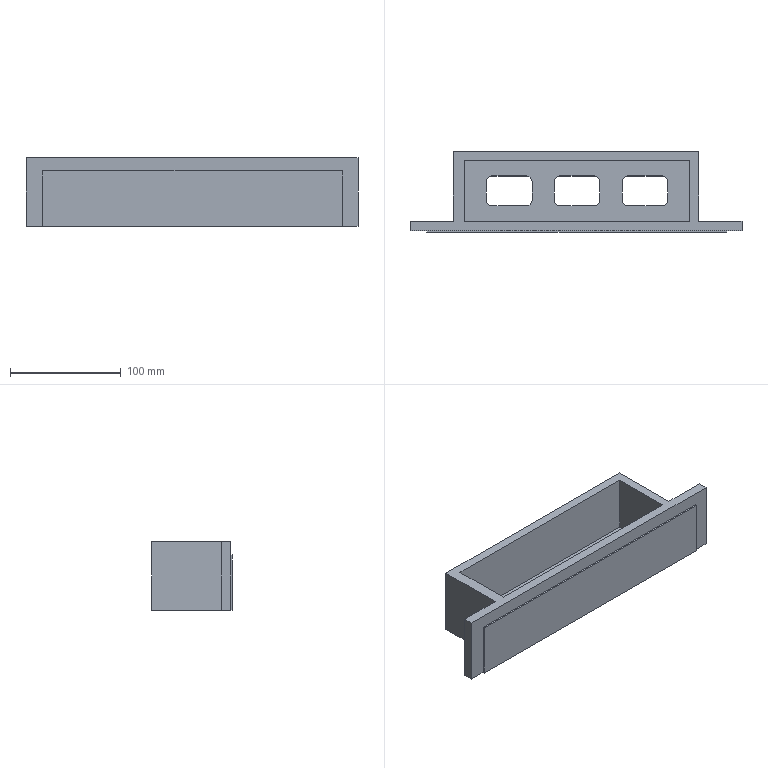Part | SolidWorks | features ICE 6, Extrusion 1, Fillet 1 | 1 solid | 43 faces | box 300 x 73 x 62 mm | volume 429281 mm3 | plane 31 | cylinder 12 | commonest cylinder face diameters 10 x12
STEP:
#1=CARTESIAN_POINT('',(-101.,5.,-21.));
#2=VERTEX_POINT('',#1);
#3=CARTESIAN_POINT('',(103.,5.,-21.));
#4=VERTEX_POINT('',#3);
#5=CARTESIAN_POINT('',(103.,5.,-21.));
#6=DIRECTION('',(1.,0.,0.));
#7=VECTOR('',#6,1000.);
#8=LINE('',#5,#7);
#9=EDGE_CURVE('',#2,#4,#8,.T.);
#10=ORIENTED_EDGE('',*,*,#9,.T.);
#11=CARTESIAN_POINT('',(103.,60.,-21.));
#12=VERTEX_POINT('',#11);
#13=CARTESIAN_POINT('',(103.,60.,-21.));
#14=DIRECTION('',(0.,-1.,0.));
#15=VECTOR('',#14,1000.);
#16=LINE('',#13,#15);
#17=EDGE_CURVE('',#12,#4,#16,.T.);
#18=ORIENTED_EDGE('',*,*,#17,.F.);
#19=CARTESIAN_POINT('',(-101.,60.,-21.));
#20=VERTEX_POINT('',#19);
#21=CARTESIAN_POINT('',(103.,60.,-21.));
#22=DIRECTION('',(1.,0.,0.));
#23=VECTOR('',#22,1000.);
#24=LINE('',#21,#23);
#25=EDGE_CURVE('',#20,#12,#24,.T.);
#26=ORIENTED_EDGE('',*,*,#25,.F.);
#27=CARTESIAN_POINT('',(-101.,60.,-21.));
#28=DIRECTION('',(0.,-1.,0.));
#29=VECTOR('',#28,1000.);
#30=LINE('',#27,#29);
#31=EDGE_CURVE('',#20,#2,#30,.T.);
#32=ORIENTED_EDGE('',*,*,#31,.T.);
#33=EDGE_LOOP('',(#10,#18,#26,#32));
#34=FACE_OUTER_BOUND('',#33,.T.);
#35=CARTESIAN_POINT('',(78.,46.,-21.));
#36=VERTEX_POINT('',#35);
#37=CARTESIAN_POINT('',(46.667,46.,-21.));
#38=VERTEX_POINT('',#37);
#39=CARTESIAN_POINT('',(41.667,46.,-21.));
#40=DIRECTION('',(-1.,0.,0.));
#41=VECTOR('',#40,1000.);
#42=LINE('',#39,#41);
#43=EDGE_CURVE('',#36,#38,#42,.T.);
#44=ORIENTED_EDGE('',*,*,#43,.F.);
#45=CARTESIAN_POINT('',(83.,41.,-21.));
#46=VERTEX_POINT('',#45);
#47=CARTESIAN_POINT('',(78.,41.,-21.));
#48=DIRECTION('',(0.,0.,-1.));
#49=DIRECTION('',(-1.,0.,0.));
#50=AXIS2_PLACEMENT_3D('',#47,#48,#49);
#51=CIRCLE('',#50,5.);
#52=EDGE_CURVE('',#36,#46,#51,.T.);
#53=ORIENTED_EDGE('',*,*,#52,.T.);
#54=CARTESIAN_POINT('',(83.,24.,-21.));
#55=VERTEX_POINT('',#54);
#56=CARTESIAN_POINT('',(83.,19.,-21.));
#57=DIRECTION('',(0.,1.,0.));
#58=VECTOR('',#57,1000.);
#59=LINE('',#56,#58);
#60=EDGE_CURVE('',#55,#46,#59,.T.);
#61=ORIENTED_EDGE('',*,*,#60,.F.);
#62=CARTESIAN_POINT('',(78.,19.,-21.));
#63=VERTEX_POINT('',#62);
#64=CARTESIAN_POINT('',(78.,24.,-21.));
#65=DIRECTION('',(0.,0.,-1.));
#66=DIRECTION('',(-1.,0.,0.));
#67=AXIS2_PLACEMENT_3D('',#64,#65,#66);
#68=CIRCLE('',#67,5.);
#69=EDGE_CURVE('',#55,#63,#68,.T.);
#70=ORIENTED_EDGE('',*,*,#69,.T.);
#71=CARTESIAN_POINT('',(46.667,19.,-21.));
#72=VERTEX_POINT('',#71);
#73=CARTESIAN_POINT('',(41.667,19.,-21.));
#74=DIRECTION('',(1.,0.,0.));
#75=VECTOR('',#74,1000.);
#76=LINE('',#73,#75);
#77=EDGE_CURVE('',#72,#63,#76,.T.);
#78=ORIENTED_EDGE('',*,*,#77,.F.);
#79=CARTESIAN_POINT('',(41.667,24.,-21.));
#80=VERTEX_POINT('',#79);
#81=CARTESIAN_POINT('',(46.667,24.,-21.));
#82=DIRECTION('',(0.,0.,-1.));
#83=DIRECTION('',(-1.,0.,0.));
#84=AXIS2_PLACEMENT_3D('',#81,#82,#83);
#85=CIRCLE('',#84,5.);
#86=EDGE_CURVE('',#72,#80,#85,.T.);
#87=ORIENTED_EDGE('',*,*,#86,.T.);
#88=CARTESIAN_POINT('',(41.667,41.,-21.));
#89=VERTEX_POINT('',#88);
#90=CARTESIAN_POINT('',(41.667,19.,-21.));
#91=DIRECTION('',(0.,-1.,0.));
#92=VECTOR('',#91,1000.);
#93=LINE('',#90,#92);
#94=EDGE_CURVE('',#89,#80,#93,.T.);
#95=ORIENTED_EDGE('',*,*,#94,.F.);
#96=CARTESIAN_POINT('',(46.667,41.,-21.));
#97=DIRECTION('',(0.,0.,-1.));
#98=DIRECTION('',(-1.,0.,0.));
#99=AXIS2_PLACEMENT_3D('',#96,#97,#98);
#100=CIRCLE('',#99,5.);
#101=EDGE_CURVE('',#89,#38,#100,.T.);
#102=ORIENTED_EDGE('',*,*,#101,.T.);
#103=EDGE_LOOP('',(#44,#53,#61,#70,#78,#87,#95,#102));
#104=FACE_BOUND('',#103,.T.);
#105=CARTESIAN_POINT('',(-44.667,46.,-21.));
#106=VERTEX_POINT('',#105);
#107=CARTESIAN_POINT('',(-76.,46.,-21.));
#108=VERTEX_POINT('',#107);
#109=CARTESIAN_POINT('',(-81.,46.,-21.));
#110=DIRECTION('',(-1.,0.,0.));
#111=VECTOR('',#110,1000.);
#112=LINE('',#109,#111);
#113=EDGE_CURVE('',#106,#108,#112,.T.);
#114=ORIENTED_EDGE('',*,*,#113,.F.);
#115=CARTESIAN_POINT('',(-39.667,41.,-21.));
#116=VERTEX_POINT('',#115);
#117=CARTESIAN_POINT('',(-44.667,41.,-21.));
#118=DIRECTION('',(0.,0.,-1.));
#119=DIRECTION('',(-1.,0.,0.));
#120=AXIS2_PLACEMENT_3D('',#117,#118,#119);
#121=CIRCLE('',#120,5.);
#122=EDGE_CURVE('',#106,#116,#121,.T.);
#123=ORIENTED_EDGE('',*,*,#122,.T.);
#124=CARTESIAN_POINT('',(-39.667,24.,-21.));
#125=VERTEX_POINT('',#124);
#126=CARTESIAN_POINT('',(-39.667,19.,-21.));
#127=DIRECTION('',(0.,1.,0.));
#128=VECTOR('',#127,1000.);
#129=LINE('',#126,#128);
#130=EDGE_CURVE('',#125,#116,#129,.T.);
#131=ORIENTED_EDGE('',*,*,#130,.F.);
#132=CARTESIAN_POINT('',(-44.667,19.,-21.));
#133=VERTEX_POINT('',#132);
#134=CARTESIAN_POINT('',(-44.667,24.,-21.));
#135=DIRECTION('',(0.,0.,-1.));
#136=DIRECTION('',(-1.,0.,0.));
#137=AXIS2_PLACEMENT_3D('',#134,#135,#136);
#138=CIRCLE('',#137,5.);
#139=EDGE_CURVE('',#125,#133,#138,.T.);
#140=ORIENTED_EDGE('',*,*,#139,.T.);
#141=CARTESIAN_POINT('',(-76.,19.,-21.));
#142=VERTEX_POINT('',#141);
#143=CARTESIAN_POINT('',(-81.,19.,-21.));
#144=DIRECTION('',(1.,0.,0.));
#145=VECTOR('',#144,1000.);
#146=LINE('',#143,#145);
#147=EDGE_CURVE('',#142,#133,#146,.T.);
#148=ORIENTED_EDGE('',*,*,#147,.F.);
#149=CARTESIAN_POINT('',(-81.,24.,-21.));
#150=VERTEX_POINT('',#149);
#151=CARTESIAN_POINT('',(-76.,24.,-21.));
#152=DIRECTION('',(0.,0.,-1.));
#153=DIRECTION('',(-1.,0.,0.));
#154=AXIS2_PLACEMENT_3D('',#151,#152,#153);
#155=CIRCLE('',#154,5.);
#156=EDGE_CURVE('',#142,#150,#155,.T.);
#157=ORIENTED_EDGE('',*,*,#156,.T.);
#158=CARTESIAN_POINT('',(-81.,41.,-21.));
#159=VERTEX_POINT('',#158);
#160=CARTESIAN_POINT('',(-81.,19.,-21.));
#161=DIRECTION('',(0.,-1.,0.));
#162=VECTOR('',#161,1000.);
#163=LINE('',#160,#162);
#164=EDGE_CURVE('',#159,#150,#163,.T.);
#165=ORIENTED_EDGE('',*,*,#164,.F.);
#166=CARTESIAN_POINT('',(-76.,41.,-21.));
#167=DIRECTION('',(0.,0.,-1.));
#168=DIRECTION('',(-1.,0.,0.));
#169=AXIS2_PLACEMENT_3D('',#166,#167,#168);
#170=CIRCLE('',#169,5.);
#171=EDGE_CURVE('',#159,#108,#170,.T.);
#172=ORIENTED_EDGE('',*,*,#171,.T.);
#173=EDGE_LOOP('',(#114,#123,#131,#140,#148,#157,#165,#172));
#174=FACE_BOUND('',#173,.T.);
#175=CARTESIAN_POINT('',(21.667,24.,-21.));
#176=VERTEX_POINT('',#175);
#177=CARTESIAN_POINT('',(21.667,41.,-21.));
#178=VERTEX_POINT('',#177);
#179=CARTESIAN_POINT('',(21.667,19.,-21.));
#180=DIRECTION('',(0.,1.,0.));
#181=VECTOR('',#180,1000.);
#182=LINE('',#179,#181);
#183=EDGE_CURVE('',#176,#178,#182,.T.);
#184=ORIENTED_EDGE('',*,*,#183,.F.);
#185=CARTESIAN_POINT('',(16.667,19.,-21.));
#186=VERTEX_POINT('',#185);
#187=CARTESIAN_POINT('',(16.667,24.,-21.));
#188=DIRECTION('',(0.,0.,-1.));
#189=DIRECTION('',(-1.,0.,0.));
#190=AXIS2_PLACEMENT_3D('',#187,#188,#189);
#191=CIRCLE('',#190,5.);
#192=EDGE_CURVE('',#176,#186,#191,.T.);
#193=ORIENTED_EDGE('',*,*,#192,.T.);
#194=CARTESIAN_POINT('',(-14.667,19.,-21.));
#195=VERTEX_POINT('',#194);
#196=CARTESIAN_POINT('',(-19.667,19.,-21.));
#197=DIRECTION('',(1.,0.,0.));
#198=VECTOR('',#197,1000.);
#199=LINE('',#196,#198);
#200=EDGE_CURVE('',#195,#186,#199,.T.);
#201=ORIENTED_EDGE('',*,*,#200,.F.);
#202=CARTESIAN_POINT('',(-19.667,24.,-21.));
#203=VERTEX_POINT('',#202);
#204=CARTESIAN_POINT('',(-14.667,24.,-21.));
#205=DIRECTION('',(0.,0.,-1.));
#206=DIRECTION('',(-1.,0.,0.));
#207=AXIS2_PLACEMENT_3D('',#204,#205,#206);
#208=CIRCLE('',#207,5.);
#209=EDGE_CURVE('',#195,#203,#208,.T.);
#210=ORIENTED_EDGE('',*,*,#209,.T.);
#211=CARTESIAN_POINT('',(-19.667,41.,-21.));
#212=VERTEX_POINT('',#211);
#213=CARTESIAN_POINT('',(-19.667,19.,-21.));
#214=DIRECTION('',(0.,-1.,0.));
#215=VECTOR('',#214,1000.);
#216=LINE('',#213,#215);
#217=EDGE_CURVE('',#212,#203,#216,.T.);
#218=ORIENTED_EDGE('',*,*,#217,.F.);
#219=CARTESIAN_POINT('',(-14.667,46.,-21.));
#220=VERTEX_POINT('',#219);
#221=CARTESIAN_POINT('',(-14.667,41.,-21.));
#222=DIRECTION('',(0.,0.,-1.));
#223=DIRECTION('',(-1.,0.,0.));
#224=AXIS2_PLACEMENT_3D('',#221,#222,#223);
#225=CIRCLE('',#224,5.);
#226=EDGE_CURVE('',#212,#220,#225,.T.);
#227=ORIENTED_EDGE('',*,*,#226,.T.);
#228=CARTESIAN_POINT('',(16.667,46.,-21.));
#229=VERTEX_POINT('',#228);
#230=CARTESIAN_POINT('',(-19.667,46.,-21.));
#231=DIRECTION('',(-1.,0.,0.));
#232=VECTOR('',#231,1000.);
#233=LINE('',#230,#232);
#234=EDGE_CURVE('',#229,#220,#233,.T.);
#235=ORIENTED_EDGE('',*,*,#234,.F.);
#236=CARTESIAN_POINT('',(16.667,41.,-21.));
#237=DIRECTION('',(0.,0.,-1.));
#238=DIRECTION('',(-1.,0.,0.));
#239=AXIS2_PLACEMENT_3D('',#236,#237,#238);
#240=CIRCLE('',#239,5.);
#241=EDGE_CURVE('',#229,#178,#240,.T.);
#242=ORIENTED_EDGE('',*,*,#241,.T.);
#243=EDGE_LOOP('',(#184,#193,#201,#210,#218,#227,#235,#242));
#244=FACE_BOUND('',#243,.T.);
#245=CARTESIAN_POINT('',(103.,60.,-21.));
#246=DIRECTION('',(0.,0.,-1.));
#247=DIRECTION('',(-1.,0.,0.));
#248=AXIS2_PLACEMENT_3D('',#245,#246,#247);
#249=PLANE('',#248);
#250=ADVANCED_FACE('',(#34,#104,#174,#244),#249,.F.);
#251=CARTESIAN_POINT('',(-111.,5.,-31.));
#252=VERTEX_POINT('',#251);
#253=CARTESIAN_POINT('',(-111.,5.,31.));
#254=VERTEX_POINT('',#253);
#255=CARTESIAN_POINT('',(-111.,5.,31.));
#256=DIRECTION('',(0.,0.,1.));
#257=VECTOR('',#256,1000.);
#258=LINE('',#255,#257);
#259=EDGE_CURVE('',#252,#254,#258,.T.);
#260=ORIENTED_EDGE('',*,*,#259,.F.);
#261=CARTESIAN_POINT('',(-150.,5.,-31.));
#262=VERTEX_POINT('',#261);
#263=CARTESIAN_POINT('',(-150.,5.,-31.));
#264=DIRECTION('',(-1.,0.,0.));
#265=VECTOR('',#264,1000.);
#266=LINE('',#263,#265);
#267=EDGE_CURVE('',#252,#262,#266,.T.);
#268=ORIENTED_EDGE('',*,*,#267,.T.);
#269=CARTESIAN_POINT('',(-150.,5.,31.));
#270=VERTEX_POINT('',#269);
#271=CARTESIAN_POINT('',(-150.,5.,31.));
#272=DIRECTION('',(0.,0.,1.));
#273=VECTOR('',#272,1000.);
#274=LINE('',#271,#273);
#275=EDGE_CURVE('',#262,#270,#274,.T.);
#276=ORIENTED_EDGE('',*,*,#275,.T.);
#277=CARTESIAN_POINT('',(-150.,5.,31.));
#278=DIRECTION('',(1.,0.,0.));
#279=VECTOR('',#278,1000.);
#280=LINE('',#277,#279);
#281=EDGE_CURVE('',#270,#254,#280,.T.);
#282=ORIENTED_EDGE('',*,*,#281,.T.);
#283=EDGE_LOOP('',(#260,#268,#276,#282));
#284=FACE_OUTER_BOUND('',#283,.T.);
#285=CARTESIAN_POINT('',(0.,5.,0.));
#286=DIRECTION('',(0.,-1.,0.));
#287=DIRECTION('',(0.,0.,-1.));
#288=AXIS2_PLACEMENT_3D('',#285,#286,#287);
#289=PLANE('',#288);
#290=ADVANCED_FACE('',(#284),#289,.F.);
#291=CARTESIAN_POINT('',(111.,5.,31.));
#292=VERTEX_POINT('',#291);
#293=CARTESIAN_POINT('',(111.,5.,-31.));
#294=VERTEX_POINT('',#293);
#295=CARTESIAN_POINT('',(111.,5.,-31.));
#296=DIRECTION('',(0.,0.,-1.));
#297=VECTOR('',#296,1000.);
#298=LINE('',#295,#297);
#299=EDGE_CURVE('',#292,#294,#298,.T.);
#300=ORIENTED_EDGE('',*,*,#299,.F.);
#301=CARTESIAN_POINT('',(150.,5.,31.));
#302=VERTEX_POINT('',#301);
#303=CARTESIAN_POINT('',(-150.,5.,31.));
#304=DIRECTION('',(1.,0.,0.));
#305=VECTOR('',#304,1000.);
#306=LINE('',#303,#305);
#307=EDGE_CURVE('',#292,#302,#306,.T.);
#308=ORIENTED_EDGE('',*,*,#307,.T.);
#309=CARTESIAN_POINT('',(150.,5.,-31.));
#310=VERTEX_POINT('',#309);
#311=CARTESIAN_POINT('',(150.,5.,31.));
#312=DIRECTION('',(0.,0.,-1.));
#313=VECTOR('',#312,1000.);
#314=LINE('',#311,#313);
#315=EDGE_CURVE('',#302,#310,#314,.T.);
#316=ORIENTED_EDGE('',*,*,#315,.T.);
#317=CARTESIAN_POINT('',(-150.,5.,-31.));
#318=DIRECTION('',(-1.,0.,0.));
#319=VECTOR('',#318,1000.);
#320=LINE('',#317,#319);
#321=EDGE_CURVE('',#310,#294,#320,.T.);
#322=ORIENTED_EDGE('',*,*,#321,.T.);
#323=EDGE_LOOP('',(#300,#308,#316,#322));
#324=FACE_OUTER_BOUND('',#323,.T.);
#325=CARTESIAN_POINT('',(0.,5.,0.));
#326=DIRECTION('',(0.,-1.,0.));
#327=DIRECTION('',(0.,0.,-1.));
#328=AXIS2_PLACEMENT_3D('',#325,#326,#327);
#329=PLANE('',#328);
#330=ADVANCED_FACE('',(#324),#329,.F.);
#331=CARTESIAN_POINT('',(103.,5.,31.));
#332=VERTEX_POINT('',#331);
#333=CARTESIAN_POINT('',(103.,5.,31.));
#334=DIRECTION('',(0.,0.,1.));
#335=VECTOR('',#334,1000.);
#336=LINE('',#333,#335);
#337=EDGE_CURVE('',#4,#332,#336,.T.);
#338=ORIENTED_EDGE('',*,*,#337,.F.);
#339=ORIENTED_EDGE('',*,*,#9,.F.);
#340=CARTESIAN_POINT('',(-101.,5.,31.));
#341=VERTEX_POINT('',#340);
#342=CARTESIAN_POINT('',(-101.,5.,-21.));
#343=DIRECTION('',(0.,0.,-1.));
#344=VECTOR('',#343,1000.);
#345=LINE('',#342,#344);
#346=EDGE_CURVE('',#341,#2,#345,.T.);
#347=ORIENTED_EDGE('',*,*,#346,.F.);
#348=CARTESIAN_POINT('',(-150.,5.,31.));
#349=DIRECTION('',(1.,0.,0.));
#350=VECTOR('',#349,1000.);
#351=LINE('',#348,#350);
#352=EDGE_CURVE('',#341,#332,#351,.T.);
#353=ORIENTED_EDGE('',*,*,#352,.T.);
#354=EDGE_LOOP('',(#338,#339,#347,#353));
#355=FACE_OUTER_BOUND('',#354,.T.);
#356=CARTESIAN_POINT('',(0.,5.,0.));
#357=DIRECTION('',(0.,-1.,0.));
#358=DIRECTION('',(0.,0.,-1.));
#359=AXIS2_PLACEMENT_3D('',#356,#357,#358);
#360=PLANE('',#359);
#361=ADVANCED_FACE('',(#355),#360,.F.);
#362=CARTESIAN_POINT('',(-150.,-3.5,31.));
#363=VERTEX_POINT('',#362);
#364=CARTESIAN_POINT('',(-150.,-3.5,-31.));
#365=VERTEX_POINT('',#364);
#366=CARTESIAN_POINT('',(-150.,-3.5,31.));
#367=DIRECTION('',(0.,0.,-1.));
#368=VECTOR('',#367,1000.);
#369=LINE('',#366,#368);
#370=EDGE_CURVE('',#363,#365,#369,.T.);
#371=ORIENTED_EDGE('',*,*,#370,.F.);
#372=CARTESIAN_POINT('',(-150.,5.,31.));
#373=DIRECTION('',(0.,-1.,0.));
#374=VECTOR('',#373,1000.);
#375=LINE('',#372,#374);
#376=EDGE_CURVE('',#270,#363,#375,.T.);
#377=ORIENTED_EDGE('',*,*,#376,.F.);
#378=ORIENTED_EDGE('',*,*,#275,.F.);
#379=CARTESIAN_POINT('',(-150.,5.,-31.));
#380=DIRECTION('',(0.,-1.,0.));
#381=VECTOR('',#380,1000.);
#382=LINE('',#379,#381);
#383=EDGE_CURVE('',#262,#365,#382,.T.);
#384=ORIENTED_EDGE('',*,*,#383,.T.);
#385=EDGE_LOOP('',(#371,#377,#378,#384));
#386=FACE_OUTER_BOUND('',#385,.T.);
#387=CARTESIAN_POINT('',(-150.,5.,31.));
#388=DIRECTION('',(1.,0.,0.));
#389=DIRECTION('',(0.,0.,-1.));
#390=AXIS2_PLACEMENT_3D('',#387,#388,#389);
#391=PLANE('',#390);
#392=ADVANCED_FACE('',(#386),#391,.F.);
#393=CARTESIAN_POINT('',(-101.,60.,31.));
#394=VERTEX_POINT('',#393);
#395=CARTESIAN_POINT('',(-101.,60.,31.));
#396=DIRECTION('',(0.,-1.,0.));
#397=VECTOR('',#396,1000.);
#398=LINE('',#395,#397);
#399=EDGE_CURVE('',#394,#341,#398,.T.);
#400=ORIENTED_EDGE('',*,*,#399,.F.);
#401=CARTESIAN_POINT('',(103.,60.,31.));
#402=VERTEX_POINT('',#401);
#403=CARTESIAN_POINT('',(-111.,60.,31.));
#404=DIRECTION('',(1.,0.,0.));
#405=VECTOR('',#404,1000.);
#406=LINE('',#403,#405);
#407=EDGE_CURVE('',#394,#402,#406,.T.);
#408=ORIENTED_EDGE('',*,*,#407,.T.);
#409=CARTESIAN_POINT('',(103.,60.,31.));
#410=DIRECTION('',(0.,-1.,0.));
#411=VECTOR('',#410,1000.);
#412=LINE('',#409,#411);
#413=EDGE_CURVE('',#402,#332,#412,.T.);
#414=ORIENTED_EDGE('',*,*,#413,.T.);
#415=ORIENTED_EDGE('',*,*,#352,.F.);
#416=EDGE_LOOP('',(#400,#408,#414,#415));
#417=FACE_BOUND('',#416,.T.);
#418=ORIENTED_EDGE('',*,*,#376,.T.);
#419=CARTESIAN_POINT('',(150.,-3.5,31.));
#420=VERTEX_POINT('',#419);
#421=CARTESIAN_POINT('',(-148.121,-3.5,31.));
#422=DIRECTION('',(-1.,0.,0.));
#423=VECTOR('',#422,1000.);
#424=LINE('',#421,#423);
#425=EDGE_CURVE('',#420,#363,#424,.T.);
#426=ORIENTED_EDGE('',*,*,#425,.F.);
#427=CARTESIAN_POINT('',(150.,5.,31.));
#428=DIRECTION('',(0.,-1.,0.));
#429=VECTOR('',#428,1000.);
#430=LINE('',#427,#429);
#431=EDGE_CURVE('',#302,#420,#430,.T.);
#432=ORIENTED_EDGE('',*,*,#431,.F.);
#433=ORIENTED_EDGE('',*,*,#307,.F.);
#434=CARTESIAN_POINT('',(111.,68.,31.));
#435=VERTEX_POINT('',#434);
#436=CARTESIAN_POINT('',(111.,60.,31.));
#437=DIRECTION('',(0.,-1.,0.));
#438=VECTOR('',#437,1000.);
#439=LINE('',#436,#438);
#440=EDGE_CURVE('',#435,#292,#439,.T.);
#441=ORIENTED_EDGE('',*,*,#440,.F.);
#442=CARTESIAN_POINT('',(-111.,68.,31.));
#443=VERTEX_POINT('',#442);
#444=CARTESIAN_POINT('',(-111.,68.,31.));
#445=DIRECTION('',(1.,0.,0.));
#446=VECTOR('',#445,1000.);
#447=LINE('',#444,#446);
#448=EDGE_CURVE('',#443,#435,#447,.T.);
#449=ORIENTED_EDGE('',*,*,#448,.F.);
#450=CARTESIAN_POINT('',(-111.,60.,31.));
#451=DIRECTION('',(0.,-1.,0.));
#452=VECTOR('',#451,1000.);
#453=LINE('',#450,#452);
#454=EDGE_CURVE('',#443,#254,#453,.T.);
#455=ORIENTED_EDGE('',*,*,#454,.T.);
#456=ORIENTED_EDGE('',*,*,#281,.F.);
#457=EDGE_LOOP('',(#418,#426,#432,#433,#441,#449,#455,#456));
#458=FACE_OUTER_BOUND('',#457,.T.);
#459=CARTESIAN_POINT('',(-150.,5.,31.));
#460=DIRECTION('',(0.,0.,-1.));
#461=DIRECTION('',(-1.,0.,0.));
#462=AXIS2_PLACEMENT_3D('',#459,#460,#461);
#463=PLANE('',#462);
#464=ADVANCED_FACE('',(#417,#458),#463,.F.);
#465=CARTESIAN_POINT('',(150.,-3.5,-31.));
#466=VERTEX_POINT('',#465);
#467=CARTESIAN_POINT('',(150.,-3.5,19.));
#468=DIRECTION('',(0.,0.,1.));
#469=VECTOR('',#468,1000.);
#470=LINE('',#467,#469);
#471=EDGE_CURVE('',#466,#420,#470,.T.);
#472=ORIENTED_EDGE('',*,*,#471,.F.);
#473=CARTESIAN_POINT('',(150.,5.,-31.));
#474=DIRECTION('',(0.,-1.,0.));
#475=VECTOR('',#474,1000.);
#476=LINE('',#473,#475);
#477=EDGE_CURVE('',#310,#466,#476,.T.);
#478=ORIENTED_EDGE('',*,*,#477,.F.);
#479=ORIENTED_EDGE('',*,*,#315,.F.);
#480=ORIENTED_EDGE('',*,*,#431,.T.);
#481=EDGE_LOOP('',(#472,#478,#479,#480));
#482=FACE_OUTER_BOUND('',#481,.T.);
#483=CARTESIAN_POINT('',(150.,5.,31.));
#484=DIRECTION('',(-1.,0.,0.));
#485=DIRECTION('',(0.,0.,1.));
#486=AXIS2_PLACEMENT_3D('',#483,#484,#485);
#487=PLANE('',#486);
#488=ADVANCED_FACE('',(#482),#487,.F.);
#489=CARTESIAN_POINT('',(-44.667,19.,-31.));
#490=VERTEX_POINT('',#489);
#491=CARTESIAN_POINT('',(-76.,19.,-31.));
#492=VERTEX_POINT('',#491);
#493=CARTESIAN_POINT('',(-81.,19.,-31.));
#494=DIRECTION('',(-1.,0.,0.));
#495=VECTOR('',#494,1000.);
#496=LINE('',#493,#495);
#497=EDGE_CURVE('',#490,#492,#496,.T.);
#498=ORIENTED_EDGE('',*,*,#497,.F.);
#499=CARTESIAN_POINT('',(-39.667,24.,-31.));
#500=VERTEX_POINT('',#499);
#501=CARTESIAN_POINT('',(-44.667,24.,-31.));
#502=DIRECTION('',(0.,0.,1.));
#503=DIRECTION('',(1.,0.,0.));
#504=AXIS2_PLACEMENT_3D('',#501,#502,#503);
#505=CIRCLE('',#504,5.);
#506=EDGE_CURVE('',#490,#500,#505,.T.);
#507=ORIENTED_EDGE('',*,*,#506,.T.);
#508=CARTESIAN_POINT('',(-39.667,41.,-31.));
#509=VERTEX_POINT('',#508);
#510=CARTESIAN_POINT('',(-39.667,19.,-31.));
#511=DIRECTION('',(0.,-1.,0.));
#512=VECTOR('',#511,1000.);
#513=LINE('',#510,#512);
#514=EDGE_CURVE('',#509,#500,#513,.T.);
#515=ORIENTED_EDGE('',*,*,#514,.F.);
#516=CARTESIAN_POINT('',(-44.667,46.,-31.));
#517=VERTEX_POINT('',#516);
#518=CARTESIAN_POINT('',(-44.667,41.,-31.));
#519=DIRECTION('',(0.,0.,1.));
#520=DIRECTION('',(1.,0.,0.));
#521=AXIS2_PLACEMENT_3D('',#518,#519,#520);
#522=CIRCLE('',#521,5.);
#523=EDGE_CURVE('',#509,#517,#522,.T.);
#524=ORIENTED_EDGE('',*,*,#523,.T.);
#525=CARTESIAN_POINT('',(-76.,46.,-31.));
#526=VERTEX_POINT('',#525);
#527=CARTESIAN_POINT('',(-81.,46.,-31.));
#528=DIRECTION('',(1.,0.,0.));
#529=VECTOR('',#528,1000.);
#530=LINE('',#527,#529);
#531=EDGE_CURVE('',#526,#517,#530,.T.);
#532=ORIENTED_EDGE('',*,*,#531,.F.);
#533=CARTESIAN_POINT('',(-81.,41.,-31.));
#534=VERTEX_POINT('',#533);
#535=CARTESIAN_POINT('',(-76.,41.,-31.));
#536=DIRECTION('',(0.,0.,1.));
#537=DIRECTION('',(1.,0.,0.));
#538=AXIS2_PLACEMENT_3D('',#535,#536,#537);
#539=CIRCLE('',#538,5.);
#540=EDGE_CURVE('',#526,#534,#539,.T.);
#541=ORIENTED_EDGE('',*,*,#540,.T.);
#542=CARTESIAN_POINT('',(-81.,24.,-31.));
#543=VERTEX_POINT('',#542);
#544=CARTESIAN_POINT('',(-81.,19.,-31.));
#545=DIRECTION('',(0.,1.,0.));
#546=VECTOR('',#545,1000.);
#547=LINE('',#544,#546);
#548=EDGE_CURVE('',#543,#534,#547,.T.);
#549=ORIENTED_EDGE('',*,*,#548,.F.);
#550=CARTESIAN_POINT('',(-76.,24.,-31.));
#551=DIRECTION('',(0.,0.,1.));
#552=DIRECTION('',(1.,0.,0.));
#553=AXIS2_PLACEMENT_3D('',#550,#551,#552);
#554=CIRCLE('',#553,5.);
#555=EDGE_CURVE('',#543,#492,#554,.T.);
#556=ORIENTED_EDGE('',*,*,#555,.T.);
#557=EDGE_LOOP('',(#498,#507,#515,#524,#532,#541,#549,#556));
#558=FACE_BOUND('',#557,.T.);
#559=CARTESIAN_POINT('',(78.,19.,-31.));
#560=VERTEX_POINT('',#559);
#561=CARTESIAN_POINT('',(46.667,19.,-31.));
#562=VERTEX_POINT('',#561);
#563=CARTESIAN_POINT('',(41.667,19.,-31.));
#564=DIRECTION('',(-1.,0.,0.));
#565=VECTOR('',#564,1000.);
#566=LINE('',#563,#565);
#567=EDGE_CURVE('',#560,#562,#566,.T.);
#568=ORIENTED_EDGE('',*,*,#567,.F.);
#569=CARTESIAN_POINT('',(83.,24.,-31.));
#570=VERTEX_POINT('',#569);
#571=CARTESIAN_POINT('',(78.,24.,-31.));
#572=DIRECTION('',(0.,0.,1.));
#573=DIRECTION('',(1.,0.,0.));
#574=AXIS2_PLACEMENT_3D('',#571,#572,#573);
#575=CIRCLE('',#574,5.);
#576=EDGE_CURVE('',#560,#570,#575,.T.);
#577=ORIENTED_EDGE('',*,*,#576,.T.);
#578=CARTESIAN_POINT('',(83.,41.,-31.));
#579=VERTEX_POINT('',#578);
#580=CARTESIAN_POINT('',(83.,19.,-31.));
#581=DIRECTION('',(0.,-1.,0.));
#582=VECTOR('',#581,1000.);
#583=LINE('',#580,#582);
#584=EDGE_CURVE('',#579,#570,#583,.T.);
#585=ORIENTED_EDGE('',*,*,#584,.F.);
#586=CARTESIAN_POINT('',(78.,46.,-31.));
#587=VERTEX_POINT('',#586);
#588=CARTESIAN_POINT('',(78.,41.,-31.));
#589=DIRECTION('',(0.,0.,1.));
#590=DIRECTION('',(1.,0.,0.));
#591=AXIS2_PLACEMENT_3D('',#588,#589,#590);
#592=CIRCLE('',#591,5.);
#593=EDGE_CURVE('',#579,#587,#592,.T.);
#594=ORIENTED_EDGE('',*,*,#593,.T.);
#595=CARTESIAN_POINT('',(46.667,46.,-31.));
#596=VERTEX_POINT('',#595);
#597=CARTESIAN_POINT('',(41.667,46.,-31.));
#598=DIRECTION('',(1.,0.,0.));
#599=VECTOR('',#598,1000.);
#600=LINE('',#597,#599);
#601=EDGE_CURVE('',#596,#587,#600,.T.);
#602=ORIENTED_EDGE('',*,*,#601,.F.);
#603=CARTESIAN_POINT('',(41.667,41.,-31.));
#604=VERTEX_POINT('',#603);
#605=CARTESIAN_POINT('',(46.667,41.,-31.));
#606=DIRECTION('',(0.,0.,1.));
#607=DIRECTION('',(1.,0.,0.));
#608=AXIS2_PLACEMENT_3D('',#605,#606,#607);
#609=CIRCLE('',#608,5.);
#610=EDGE_CURVE('',#596,#604,#609,.T.);
#611=ORIENTED_EDGE('',*,*,#610,.T.);
#612=CARTESIAN_POINT('',(41.667,24.,-31.));
#613=VERTEX_POINT('',#612);
#614=CARTESIAN_POINT('',(41.667,19.,-31.));
#615=DIRECTION('',(0.,1.,0.));
#616=VECTOR('',#615,1000.);
#617=LINE('',#614,#616);
#618=EDGE_CURVE('',#613,#604,#617,.T.);
#619=ORIENTED_EDGE('',*,*,#618,.F.);
#620=CARTESIAN_POINT('',(46.667,24.,-31.));
#621=DIRECTION('',(0.,0.,1.));
#622=DIRECTION('',(1.,0.,0.));
#623=AXIS2_PLACEMENT_3D('',#620,#621,#622);
#624=CIRCLE('',#623,5.);
#625=EDGE_CURVE('',#613,#562,#624,.T.);
#626=ORIENTED_EDGE('',*,*,#625,.T.);
#627=EDGE_LOOP('',(#568,#577,#585,#594,#602,#611,#619,#626));
#628=FACE_BOUND('',#627,.T.);
#629=CARTESIAN_POINT('',(16.667,19.,-31.));
#630=VERTEX_POINT('',#629);
#631=CARTESIAN_POINT('',(-14.667,19.,-31.));
#632=VERTEX_POINT('',#631);
#633=CARTESIAN_POINT('',(-19.667,19.,-31.));
#634=DIRECTION('',(-1.,0.,0.));
#635=VECTOR('',#634,1000.);
#636=LINE('',#633,#635);
#637=EDGE_CURVE('',#630,#632,#636,.T.);
#638=ORIENTED_EDGE('',*,*,#637,.F.);
#639=CARTESIAN_POINT('',(21.667,24.,-31.));
#640=VERTEX_POINT('',#639);
#641=CARTESIAN_POINT('',(16.667,24.,-31.));
#642=DIRECTION('',(0.,0.,1.));
#643=DIRECTION('',(1.,0.,0.));
#644=AXIS2_PLACEMENT_3D('',#641,#642,#643);
#645=CIRCLE('',#644,5.);
#646=EDGE_CURVE('',#630,#640,#645,.T.);
#647=ORIENTED_EDGE('',*,*,#646,.T.);
#648=CARTESIAN_POINT('',(21.667,41.,-31.));
#649=VERTEX_POINT('',#648);
#650=CARTESIAN_POINT('',(21.667,19.,-31.));
#651=DIRECTION('',(0.,-1.,0.));
#652=VECTOR('',#651,1000.);
#653=LINE('',#650,#652);
#654=EDGE_CURVE('',#649,#640,#653,.T.);
#655=ORIENTED_EDGE('',*,*,#654,.F.);
#656=CARTESIAN_POINT('',(16.667,46.,-31.));
#657=VERTEX_POINT('',#656);
#658=CARTESIAN_POINT('',(16.667,41.,-31.));
#659=DIRECTION('',(0.,0.,1.));
#660=DIRECTION('',(1.,0.,0.));
#661=AXIS2_PLACEMENT_3D('',#658,#659,#660);
#662=CIRCLE('',#661,5.);
#663=EDGE_CURVE('',#649,#657,#662,.T.);
#664=ORIENTED_EDGE('',*,*,#663,.T.);
#665=CARTESIAN_POINT('',(-14.667,46.,-31.));
#666=VERTEX_POINT('',#665);
#667=CARTESIAN_POINT('',(-19.667,46.,-31.));
#668=DIRECTION('',(1.,0.,0.));
#669=VECTOR('',#668,1000.);
#670=LINE('',#667,#669);
#671=EDGE_CURVE('',#666,#657,#670,.T.);
#672=ORIENTED_EDGE('',*,*,#671,.F.);
#673=CARTESIAN_POINT('',(-19.667,41.,-31.));
#674=VERTEX_POINT('',#673);
#675=CARTESIAN_POINT('',(-14.667,41.,-31.));
#676=DIRECTION('',(0.,0.,1.));
#677=DIRECTION('',(1.,0.,0.));
#678=AXIS2_PLACEMENT_3D('',#675,#676,#677);
#679=CIRCLE('',#678,5.);
#680=EDGE_CURVE('',#666,#674,#679,.T.);
#681=ORIENTED_EDGE('',*,*,#680,.T.);
#682=CARTESIAN_POINT('',(-19.667,24.,-31.));
#683=VERTEX_POINT('',#682);
#684=CARTESIAN_POINT('',(-19.667,19.,-31.));
#685=DIRECTION('',(0.,1.,0.));
#686=VECTOR('',#685,1000.);
#687=LINE('',#684,#686);
#688=EDGE_CURVE('',#683,#674,#687,.T.);
#689=ORIENTED_EDGE('',*,*,#688,.F.);
#690=CARTESIAN_POINT('',(-14.667,24.,-31.));
#691=DIRECTION('',(0.,0.,1.));
#692=DIRECTION('',(1.,0.,0.));
#693=AXIS2_PLACEMENT_3D('',#690,#691,#692);
#694=CIRCLE('',#693,5.);
#695=EDGE_CURVE('',#683,#632,#694,.T.);
#696=ORIENTED_EDGE('',*,*,#695,.T.);
#697=EDGE_LOOP('',(#638,#647,#655,#664,#672,#681,#689,#696));
#698=FACE_BOUND('',#697,.T.);
#699=CARTESIAN_POINT('',(136.,-5.,-31.));
#700=VERTEX_POINT('',#699);
#701=CARTESIAN_POINT('',(-135.,-5.,-31.));
#702=VERTEX_POINT('',#701);
#703=CARTESIAN_POINT('',(-150.,-5.,-31.));
#704=DIRECTION('',(-1.,0.,0.));
#705=VECTOR('',#704,1000.);
#706=LINE('',#703,#705);
#707=EDGE_CURVE('',#700,#702,#706,.T.);
#708=ORIENTED_EDGE('',*,*,#707,.T.);
#709=CARTESIAN_POINT('',(-135.,-3.5,-31.));
#710=VERTEX_POINT('',#709);
#711=CARTESIAN_POINT('',(-135.,-3.5,-31.));
#712=DIRECTION('',(0.,-1.,0.));
#713=VECTOR('',#712,1000.);
#714=LINE('',#711,#713);
#715=EDGE_CURVE('',#710,#702,#714,.T.);
#716=ORIENTED_EDGE('',*,*,#715,.F.);
#717=CARTESIAN_POINT('',(-150.,-3.5,-31.));
#718=DIRECTION('',(1.,0.,0.));
#719=VECTOR('',#718,1000.);
#720=LINE('',#717,#719);
#721=EDGE_CURVE('',#365,#710,#720,.T.);
#722=ORIENTED_EDGE('',*,*,#721,.F.);
#723=ORIENTED_EDGE('',*,*,#383,.F.);
#724=ORIENTED_EDGE('',*,*,#267,.F.);
#725=CARTESIAN_POINT('',(-111.,68.,-31.));
#726=VERTEX_POINT('',#725);
#727=CARTESIAN_POINT('',(-111.,60.,-31.));
#728=DIRECTION('',(0.,-1.,0.));
#729=VECTOR('',#728,1000.);
#730=LINE('',#727,#729);
#731=EDGE_CURVE('',#726,#252,#730,.T.);
#732=ORIENTED_EDGE('',*,*,#731,.F.);
#733=CARTESIAN_POINT('',(111.,68.,-31.));
#734=VERTEX_POINT('',#733);
#735=CARTESIAN_POINT('',(-111.,68.,-31.));
#736=DIRECTION('',(-1.,0.,0.));
#737=VECTOR('',#736,1000.);
#738=LINE('',#735,#737);
#739=EDGE_CURVE('',#734,#726,#738,.T.);
#740=ORIENTED_EDGE('',*,*,#739,.F.);
#741=CARTESIAN_POINT('',(111.,60.,-31.));
#742=DIRECTION('',(0.,-1.,0.));
#743=VECTOR('',#742,1000.);
#744=LINE('',#741,#743);
#745=EDGE_CURVE('',#734,#294,#744,.T.);
#746=ORIENTED_EDGE('',*,*,#745,.T.);
#747=ORIENTED_EDGE('',*,*,#321,.F.);
#748=ORIENTED_EDGE('',*,*,#477,.T.);
#749=CARTESIAN_POINT('',(136.,-3.5,-31.));
#750=VERTEX_POINT('',#749);
#751=CARTESIAN_POINT('',(150.,-3.5,-31.));
#752=DIRECTION('',(1.,0.,0.));
#753=VECTOR('',#752,1000.);
#754=LINE('',#751,#753);
#755=EDGE_CURVE('',#750,#466,#754,.T.);
#756=ORIENTED_EDGE('',*,*,#755,.F.);
#757=CARTESIAN_POINT('',(136.,-3.5,-31.));
#758=DIRECTION('',(0.,-1.,0.));
#759=VECTOR('',#758,1000.);
#760=LINE('',#757,#759);
#761=EDGE_CURVE('',#750,#700,#760,.T.);
#762=ORIENTED_EDGE('',*,*,#761,.T.);
#763=EDGE_LOOP('',(#708,#716,#722,#723,#724,#732,#740,#746,#747,#748,#756,#762));
#764=FACE_OUTER_BOUND('',#763,.T.);
#765=CARTESIAN_POINT('',(-150.,5.,-31.));
#766=DIRECTION('',(0.,0.,1.));
#767=DIRECTION('',(1.,0.,0.));
#768=AXIS2_PLACEMENT_3D('',#765,#766,#767);
#769=PLANE('',#768);
#770=ADVANCED_FACE('',(#558,#628,#698,#764),#769,.F.);
#771=CARTESIAN_POINT('',(-135.,-5.,19.));
#772=VERTEX_POINT('',#771);
#773=CARTESIAN_POINT('',(-135.,-5.,31.));
#774=DIRECTION('',(0.,0.,1.));
#775=VECTOR('',#774,1000.);
#776=LINE('',#773,#775);
#777=EDGE_CURVE('',#702,#772,#776,.T.);
#778=ORIENTED_EDGE('',*,*,#777,.F.);
#779=ORIENTED_EDGE('',*,*,#707,.F.);
#780=CARTESIAN_POINT('',(136.,-5.,19.));
#781=VERTEX_POINT('',#780);
#782=CARTESIAN_POINT('',(136.,-5.,31.));
#783=DIRECTION('',(0.,0.,-1.));
#784=VECTOR('',#783,1000.);
#785=LINE('',#782,#784);
#786=EDGE_CURVE('',#781,#700,#785,.T.);
#787=ORIENTED_EDGE('',*,*,#786,.F.);
#788=CARTESIAN_POINT('',(-148.121,-5.,19.));
#789=DIRECTION('',(1.,0.,0.));
#790=VECTOR('',#789,1000.);
#791=LINE('',#788,#790);
#792=EDGE_CURVE('',#772,#781,#791,.T.);
#793=ORIENTED_EDGE('',*,*,#792,.F.);
#794=EDGE_LOOP('',(#778,#779,#787,#793));
#795=FACE_OUTER_BOUND('',#794,.T.);
#796=CARTESIAN_POINT('',(0.,-5.,0.));
#797=DIRECTION('',(0.,-1.,0.));
#798=DIRECTION('',(0.,0.,-1.));
#799=AXIS2_PLACEMENT_3D('',#796,#797,#798);
#800=PLANE('',#799);
#801=ADVANCED_FACE('',(#795),#800,.T.);
#802=CARTESIAN_POINT('',(-135.,-3.5,19.));
#803=VERTEX_POINT('',#802);
#804=CARTESIAN_POINT('',(136.,-3.5,19.));
#805=VERTEX_POINT('',#804);
#806=CARTESIAN_POINT('',(-148.121,-3.5,19.));
#807=DIRECTION('',(1.,0.,0.));
#808=VECTOR('',#807,1000.);
#809=LINE('',#806,#808);
#810=EDGE_CURVE('',#803,#805,#809,.T.);
#811=ORIENTED_EDGE('',*,*,#810,.F.);
#812=CARTESIAN_POINT('',(-135.,-3.5,19.));
#813=DIRECTION('',(0.,-1.,0.));
#814=VECTOR('',#813,1000.);
#815=LINE('',#812,#814);
#816=EDGE_CURVE('',#803,#772,#815,.T.);
#817=ORIENTED_EDGE('',*,*,#816,.T.);
#818=ORIENTED_EDGE('',*,*,#792,.T.);
#819=CARTESIAN_POINT('',(136.,-3.5,19.));
#820=DIRECTION('',(0.,1.,0.));
#821=VECTOR('',#820,1000.);
#822=LINE('',#819,#821);
#823=EDGE_CURVE('',#781,#805,#822,.T.);
#824=ORIENTED_EDGE('',*,*,#823,.T.);
#825=EDGE_LOOP('',(#811,#817,#818,#824));
#826=FACE_OUTER_BOUND('',#825,.T.);
#827=CARTESIAN_POINT('',(-148.121,-3.5,19.));
#828=DIRECTION('',(0.,0.,-1.));
#829=DIRECTION('',(-1.,0.,0.));
#830=AXIS2_PLACEMENT_3D('',#827,#828,#829);
#831=PLANE('',#830);
#832=ADVANCED_FACE('',(#826),#831,.F.);
#833=ORIENTED_EDGE('',*,*,#425,.T.);
#834=ORIENTED_EDGE('',*,*,#370,.T.);
#835=ORIENTED_EDGE('',*,*,#721,.T.);
#836=CARTESIAN_POINT('',(-135.,-3.5,31.));
#837=DIRECTION('',(0.,0.,1.));
#838=VECTOR('',#837,1000.);
#839=LINE('',#836,#838);
#840=EDGE_CURVE('',#710,#803,#839,.T.);
#841=ORIENTED_EDGE('',*,*,#840,.T.);
#842=ORIENTED_EDGE('',*,*,#810,.T.);
#843=CARTESIAN_POINT('',(136.,-3.5,31.));
#844=DIRECTION('',(0.,0.,-1.));
#845=VECTOR('',#844,1000.);
#846=LINE('',#843,#845);
#847=EDGE_CURVE('',#805,#750,#846,.T.);
#848=ORIENTED_EDGE('',*,*,#847,.T.);
#849=ORIENTED_EDGE('',*,*,#755,.T.);
#850=ORIENTED_EDGE('',*,*,#471,.T.);
#851=EDGE_LOOP('',(#833,#834,#835,#841,#842,#848,#849,#850));
#852=FACE_OUTER_BOUND('',#851,.T.);
#853=CARTESIAN_POINT('',(0.,-3.5,0.));
#854=DIRECTION('',(0.,1.,0.));
#855=DIRECTION('',(0.,0.,1.));
#856=AXIS2_PLACEMENT_3D('',#853,#854,#855);
#857=PLANE('',#856);
#858=ADVANCED_FACE('',(#852),#857,.F.);
#859=ORIENTED_EDGE('',*,*,#786,.T.);
#860=ORIENTED_EDGE('',*,*,#761,.F.);
#861=ORIENTED_EDGE('',*,*,#847,.F.);
#862=ORIENTED_EDGE('',*,*,#823,.F.);
#863=EDGE_LOOP('',(#859,#860,#861,#862));
#864=FACE_OUTER_BOUND('',#863,.T.);
#865=CARTESIAN_POINT('',(136.,-3.5,31.));
#866=DIRECTION('',(-1.,0.,0.));
#867=DIRECTION('',(0.,0.,1.));
#868=AXIS2_PLACEMENT_3D('',#865,#866,#867);
#869=PLANE('',#868);
#870=ADVANCED_FACE('',(#864),#869,.F.);
#871=ORIENTED_EDGE('',*,*,#840,.F.);
#872=ORIENTED_EDGE('',*,*,#715,.T.);
#873=ORIENTED_EDGE('',*,*,#777,.T.);
#874=ORIENTED_EDGE('',*,*,#816,.F.);
#875=EDGE_LOOP('',(#871,#872,#873,#874));
#876=FACE_OUTER_BOUND('',#875,.T.);
#877=CARTESIAN_POINT('',(-135.,-3.5,31.));
#878=DIRECTION('',(1.,0.,0.));
#879=DIRECTION('',(0.,0.,-1.));
#880=AXIS2_PLACEMENT_3D('',#877,#878,#879);
#881=PLANE('',#880);
#882=ADVANCED_FACE('',(#876),#881,.F.);
#883=ORIENTED_EDGE('',*,*,#346,.T.);
#884=ORIENTED_EDGE('',*,*,#31,.F.);
#885=CARTESIAN_POINT('',(-101.,60.,-21.));
#886=DIRECTION('',(0.,0.,-1.));
#887=VECTOR('',#886,1000.);
#888=LINE('',#885,#887);
#889=EDGE_CURVE('',#394,#20,#888,.T.);
#890=ORIENTED_EDGE('',*,*,#889,.F.);
#891=ORIENTED_EDGE('',*,*,#399,.T.);
#892=EDGE_LOOP('',(#883,#884,#890,#891));
#893=FACE_OUTER_BOUND('',#892,.T.);
#894=CARTESIAN_POINT('',(-101.,60.,-21.));
#895=DIRECTION('',(-1.,0.,0.));
#896=DIRECTION('',(0.,0.,1.));
#897=AXIS2_PLACEMENT_3D('',#894,#895,#896);
#898=PLANE('',#897);
#899=ADVANCED_FACE('',(#893),#898,.F.);
#900=ORIENTED_EDGE('',*,*,#337,.T.);
#901=ORIENTED_EDGE('',*,*,#413,.F.);
#902=CARTESIAN_POINT('',(103.,60.,31.));
#903=DIRECTION('',(0.,0.,1.));
#904=VECTOR('',#903,1000.);
#905=LINE('',#902,#904);
#906=EDGE_CURVE('',#12,#402,#905,.T.);
#907=ORIENTED_EDGE('',*,*,#906,.F.);
#908=ORIENTED_EDGE('',*,*,#17,.T.);
#909=EDGE_LOOP('',(#900,#901,#907,#908));
#910=FACE_OUTER_BOUND('',#909,.T.);
#911=CARTESIAN_POINT('',(103.,60.,31.));
#912=DIRECTION('',(1.,0.,0.));
#913=DIRECTION('',(0.,0.,-1.));
#914=AXIS2_PLACEMENT_3D('',#911,#912,#913);
#915=PLANE('',#914);
#916=ADVANCED_FACE('',(#910),#915,.F.);
#917=ORIENTED_EDGE('',*,*,#299,.T.);
#918=ORIENTED_EDGE('',*,*,#745,.F.);
#919=CARTESIAN_POINT('',(111.,68.,31.));
#920=DIRECTION('',(0.,0.,-1.));
#921=VECTOR('',#920,1000.);
#922=LINE('',#919,#921);
#923=EDGE_CURVE('',#435,#734,#922,.T.);
#924=ORIENTED_EDGE('',*,*,#923,.F.);
#925=ORIENTED_EDGE('',*,*,#440,.T.);
#926=EDGE_LOOP('',(#917,#918,#924,#925));
#927=FACE_OUTER_BOUND('',#926,.T.);
#928=CARTESIAN_POINT('',(111.,60.,-31.));
#929=DIRECTION('',(-1.,0.,0.));
#930=DIRECTION('',(0.,0.,1.));
#931=AXIS2_PLACEMENT_3D('',#928,#929,#930);
#932=PLANE('',#931);
#933=ADVANCED_FACE('',(#927),#932,.F.);
#934=ORIENTED_EDGE('',*,*,#259,.T.);
#935=ORIENTED_EDGE('',*,*,#454,.F.);
#936=CARTESIAN_POINT('',(-111.,68.,31.));
#937=DIRECTION('',(0.,0.,1.));
#938=VECTOR('',#937,1000.);
#939=LINE('',#936,#938);
#940=EDGE_CURVE('',#726,#443,#939,.T.);
#941=ORIENTED_EDGE('',*,*,#940,.F.);
#942=ORIENTED_EDGE('',*,*,#731,.T.);
#943=EDGE_LOOP('',(#934,#935,#941,#942));
#944=FACE_OUTER_BOUND('',#943,.T.);
#945=CARTESIAN_POINT('',(-111.,60.,31.));
#946=DIRECTION('',(1.,0.,0.));
#947=DIRECTION('',(0.,0.,-1.));
#948=AXIS2_PLACEMENT_3D('',#945,#946,#947);
#949=PLANE('',#948);
#950=ADVANCED_FACE('',(#944),#949,.F.);
#951=ORIENTED_EDGE('',*,*,#940,.T.);
#952=ORIENTED_EDGE('',*,*,#448,.T.);
#953=ORIENTED_EDGE('',*,*,#923,.T.);
#954=ORIENTED_EDGE('',*,*,#739,.T.);
#955=EDGE_LOOP('',(#951,#952,#953,#954));
#956=FACE_OUTER_BOUND('',#955,.T.);
#957=CARTESIAN_POINT('',(0.,68.,0.));
#958=DIRECTION('',(0.,-1.,0.));
#959=DIRECTION('',(0.,0.,-1.));
#960=AXIS2_PLACEMENT_3D('',#957,#958,#959);
#961=PLANE('',#960);
#962=ADVANCED_FACE('',(#956),#961,.F.);
#963=ORIENTED_EDGE('',*,*,#407,.F.);
#964=ORIENTED_EDGE('',*,*,#889,.T.);
#965=ORIENTED_EDGE('',*,*,#25,.T.);
#966=ORIENTED_EDGE('',*,*,#906,.T.);
#967=EDGE_LOOP('',(#963,#964,#965,#966));
#968=FACE_OUTER_BOUND('',#967,.T.);
#969=CARTESIAN_POINT('',(0.,60.,0.));
#970=DIRECTION('',(0.,-1.,0.));
#971=DIRECTION('',(0.,0.,-1.));
#972=AXIS2_PLACEMENT_3D('',#969,#970,#971);
#973=PLANE('',#972);
#974=ADVANCED_FACE('',(#968),#973,.T.);
#975=ORIENTED_EDGE('',*,*,#60,.T.);
#976=CARTESIAN_POINT('',(83.,41.,-31.));
#977=DIRECTION('',(0.,0.,-1.));
#978=VECTOR('',#977,1000.);
#979=LINE('',#976,#978);
#980=EDGE_CURVE('',#46,#579,#979,.T.);
#981=ORIENTED_EDGE('',*,*,#980,.T.);
#982=ORIENTED_EDGE('',*,*,#584,.T.);
#983=CARTESIAN_POINT('',(83.,24.,-21.));
#984=DIRECTION('',(0.,0.,1.));
#985=VECTOR('',#984,1000.);
#986=LINE('',#983,#985);
#987=EDGE_CURVE('',#570,#55,#986,.T.);
#988=ORIENTED_EDGE('',*,*,#987,.T.);
#989=EDGE_LOOP('',(#975,#981,#982,#988));
#990=FACE_OUTER_BOUND('',#989,.T.);
#991=CARTESIAN_POINT('',(83.,19.,-31.001));
#992=DIRECTION('',(1.,0.,0.));
#993=DIRECTION('',(0.,0.,-1.));
#994=AXIS2_PLACEMENT_3D('',#991,#992,#993);
#995=PLANE('',#994);
#996=ADVANCED_FACE('',(#990),#995,.F.);
#997=ORIENTED_EDGE('',*,*,#567,.T.);
#998=CARTESIAN_POINT('',(46.667,19.,-21.));
#999=DIRECTION('',(0.,0.,1.));
#1000=VECTOR('',#999,1000.);
#1001=LINE('',#998,#1000);
#1002=EDGE_CURVE('',#562,#72,#1001,.T.);
#1003=ORIENTED_EDGE('',*,*,#1002,.T.);
#1004=ORIENTED_EDGE('',*,*,#77,.T.);
#1005=CARTESIAN_POINT('',(78.,19.,-31.));
#1006=DIRECTION('',(0.,0.,-1.));
#1007=VECTOR('',#1006,1000.);
#1008=LINE('',#1005,#1007);
#1009=EDGE_CURVE('',#63,#560,#1008,.T.);
#1010=ORIENTED_EDGE('',*,*,#1009,.T.);
#1011=EDGE_LOOP('',(#997,#1003,#1004,#1010));
#1012=FACE_OUTER_BOUND('',#1011,.T.);
#1013=CARTESIAN_POINT('',(41.667,19.,-31.001));
#1014=DIRECTION('',(0.,-1.,0.));
#1015=DIRECTION('',(0.,0.,-1.));
#1016=AXIS2_PLACEMENT_3D('',#1013,#1014,#1015);
#1017=PLANE('',#1016);
#1018=ADVANCED_FACE('',(#1012),#1017,.F.);
#1019=ORIENTED_EDGE('',*,*,#94,.T.);
#1020=CARTESIAN_POINT('',(41.667,24.,-31.));
#1021=DIRECTION('',(0.,0.,-1.));
#1022=VECTOR('',#1021,1000.);
#1023=LINE('',#1020,#1022);
#1024=EDGE_CURVE('',#80,#613,#1023,.T.);
#1025=ORIENTED_EDGE('',*,*,#1024,.T.);
#1026=ORIENTED_EDGE('',*,*,#618,.T.);
#1027=CARTESIAN_POINT('',(41.667,41.,-21.));
#1028=DIRECTION('',(0.,0.,1.));
#1029=VECTOR('',#1028,1000.);
#1030=LINE('',#1027,#1029);
#1031=EDGE_CURVE('',#604,#89,#1030,.T.);
#1032=ORIENTED_EDGE('',*,*,#1031,.T.);
#1033=EDGE_LOOP('',(#1019,#1025,#1026,#1032));
#1034=FACE_OUTER_BOUND('',#1033,.T.);
#1035=CARTESIAN_POINT('',(41.667,19.,-31.001));
#1036=DIRECTION('',(-1.,0.,0.));
#1037=DIRECTION('',(0.,0.,1.));
#1038=AXIS2_PLACEMENT_3D('',#1035,#1036,#1037);
#1039=PLANE('',#1038);
#1040=ADVANCED_FACE('',(#1034),#1039,.F.);
#1041=ORIENTED_EDGE('',*,*,#43,.T.);
#1042=CARTESIAN_POINT('',(46.667,46.,-31.));
#1043=DIRECTION('',(0.,0.,-1.));
#1044=VECTOR('',#1043,1000.);
#1045=LINE('',#1042,#1044);
#1046=EDGE_CURVE('',#38,#596,#1045,.T.);
#1047=ORIENTED_EDGE('',*,*,#1046,.T.);
#1048=ORIENTED_EDGE('',*,*,#601,.T.);
#1049=CARTESIAN_POINT('',(78.,46.,-21.));
#1050=DIRECTION('',(0.,0.,1.));
#1051=VECTOR('',#1050,1000.);
#1052=LINE('',#1049,#1051);
#1053=EDGE_CURVE('',#587,#36,#1052,.T.);
#1054=ORIENTED_EDGE('',*,*,#1053,.T.);
#1055=EDGE_LOOP('',(#1041,#1047,#1048,#1054));
#1056=FACE_OUTER_BOUND('',#1055,.T.);
#1057=CARTESIAN_POINT('',(41.667,46.,-31.001));
#1058=DIRECTION('',(0.,1.,0.));
#1059=DIRECTION('',(0.,0.,1.));
#1060=AXIS2_PLACEMENT_3D('',#1057,#1058,#1059);
#1061=PLANE('',#1060);
#1062=ADVANCED_FACE('',(#1056),#1061,.F.);
#1063=ORIENTED_EDGE('',*,*,#130,.T.);
#1064=CARTESIAN_POINT('',(-39.667,41.,-31.));
#1065=DIRECTION('',(0.,0.,-1.));
#1066=VECTOR('',#1065,1000.);
#1067=LINE('',#1064,#1066);
#1068=EDGE_CURVE('',#116,#509,#1067,.T.);
#1069=ORIENTED_EDGE('',*,*,#1068,.T.);
#1070=ORIENTED_EDGE('',*,*,#514,.T.);
#1071=CARTESIAN_POINT('',(-39.667,24.,-21.));
#1072=DIRECTION('',(0.,0.,1.));
#1073=VECTOR('',#1072,1000.);
#1074=LINE('',#1071,#1073);
#1075=EDGE_CURVE('',#500,#125,#1074,.T.);
#1076=ORIENTED_EDGE('',*,*,#1075,.T.);
#1077=EDGE_LOOP('',(#1063,#1069,#1070,#1076));
#1078=FACE_OUTER_BOUND('',#1077,.T.);
#1079=CARTESIAN_POINT('',(-39.667,19.,-31.001));
#1080=DIRECTION('',(1.,0.,0.));
#1081=DIRECTION('',(0.,0.,-1.));
#1082=AXIS2_PLACEMENT_3D('',#1079,#1080,#1081);
#1083=PLANE('',#1082);
#1084=ADVANCED_FACE('',(#1078),#1083,.F.);
#1085=ORIENTED_EDGE('',*,*,#497,.T.);
#1086=CARTESIAN_POINT('',(-76.,19.,-21.));
#1087=DIRECTION('',(0.,0.,1.));
#1088=VECTOR('',#1087,1000.);
#1089=LINE('',#1086,#1088);
#1090=EDGE_CURVE('',#492,#142,#1089,.T.);
#1091=ORIENTED_EDGE('',*,*,#1090,.T.);
#1092=ORIENTED_EDGE('',*,*,#147,.T.);
#1093=CARTESIAN_POINT('',(-44.667,19.,-31.));
#1094=DIRECTION('',(0.,0.,-1.));
#1095=VECTOR('',#1094,1000.);
#1096=LINE('',#1093,#1095);
#1097=EDGE_CURVE('',#133,#490,#1096,.T.);
#1098=ORIENTED_EDGE('',*,*,#1097,.T.);
#1099=EDGE_LOOP('',(#1085,#1091,#1092,#1098));
#1100=FACE_OUTER_BOUND('',#1099,.T.);
#1101=CARTESIAN_POINT('',(-81.,19.,-31.001));
#1102=DIRECTION('',(0.,-1.,0.));
#1103=DIRECTION('',(0.,0.,-1.));
#1104=AXIS2_PLACEMENT_3D('',#1101,#1102,#1103);
#1105=PLANE('',#1104);
#1106=ADVANCED_FACE('',(#1100),#1105,.F.);
#1107=ORIENTED_EDGE('',*,*,#164,.T.);
#1108=CARTESIAN_POINT('',(-81.,24.,-31.));
#1109=DIRECTION('',(0.,0.,-1.));
#1110=VECTOR('',#1109,1000.);
#1111=LINE('',#1108,#1110);
#1112=EDGE_CURVE('',#150,#543,#1111,.T.);
#1113=ORIENTED_EDGE('',*,*,#1112,.T.);
#1114=ORIENTED_EDGE('',*,*,#548,.T.);
#1115=CARTESIAN_POINT('',(-81.,41.,-21.));
#1116=DIRECTION('',(0.,0.,1.));
#1117=VECTOR('',#1116,1000.);
#1118=LINE('',#1115,#1117);
#1119=EDGE_CURVE('',#534,#159,#1118,.T.);
#1120=ORIENTED_EDGE('',*,*,#1119,.T.);
#1121=EDGE_LOOP('',(#1107,#1113,#1114,#1120));
#1122=FACE_OUTER_BOUND('',#1121,.T.);
#1123=CARTESIAN_POINT('',(-81.,19.,-31.001));
#1124=DIRECTION('',(-1.,0.,0.));
#1125=DIRECTION('',(0.,0.,1.));
#1126=AXIS2_PLACEMENT_3D('',#1123,#1124,#1125);
#1127=PLANE('',#1126);
#1128=ADVANCED_FACE('',(#1122),#1127,.F.);
#1129=ORIENTED_EDGE('',*,*,#113,.T.);
#1130=CARTESIAN_POINT('',(-76.,46.,-31.));
#1131=DIRECTION('',(0.,0.,-1.));
#1132=VECTOR('',#1131,1000.);
#1133=LINE('',#1130,#1132);
#1134=EDGE_CURVE('',#108,#526,#1133,.T.);
#1135=ORIENTED_EDGE('',*,*,#1134,.T.);
#1136=ORIENTED_EDGE('',*,*,#531,.T.);
#1137=CARTESIAN_POINT('',(-44.667,46.,-21.));
#1138=DIRECTION('',(0.,0.,1.));
#1139=VECTOR('',#1138,1000.);
#1140=LINE('',#1137,#1139);
#1141=EDGE_CURVE('',#517,#106,#1140,.T.);
#1142=ORIENTED_EDGE('',*,*,#1141,.T.);
#1143=EDGE_LOOP('',(#1129,#1135,#1136,#1142));
#1144=FACE_OUTER_BOUND('',#1143,.T.);
#1145=CARTESIAN_POINT('',(-81.,46.,-31.001));
#1146=DIRECTION('',(0.,1.,0.));
#1147=DIRECTION('',(0.,0.,1.));
#1148=AXIS2_PLACEMENT_3D('',#1145,#1146,#1147);
#1149=PLANE('',#1148);
#1150=ADVANCED_FACE('',(#1144),#1149,.F.);
#1151=ORIENTED_EDGE('',*,*,#183,.T.);
#1152=CARTESIAN_POINT('',(21.667,41.,-31.));
#1153=DIRECTION('',(0.,0.,-1.));
#1154=VECTOR('',#1153,1000.);
#1155=LINE('',#1152,#1154);
#1156=EDGE_CURVE('',#178,#649,#1155,.T.);
#1157=ORIENTED_EDGE('',*,*,#1156,.T.);
#1158=ORIENTED_EDGE('',*,*,#654,.T.);
#1159=CARTESIAN_POINT('',(21.667,24.,-21.));
#1160=DIRECTION('',(0.,0.,1.));
#1161=VECTOR('',#1160,1000.);
#1162=LINE('',#1159,#1161);
#1163=EDGE_CURVE('',#640,#176,#1162,.T.);
#1164=ORIENTED_EDGE('',*,*,#1163,.T.);
#1165=EDGE_LOOP('',(#1151,#1157,#1158,#1164));
#1166=FACE_OUTER_BOUND('',#1165,.T.);
#1167=CARTESIAN_POINT('',(21.667,19.,-31.001));
#1168=DIRECTION('',(1.,0.,0.));
#1169=DIRECTION('',(0.,0.,-1.));
#1170=AXIS2_PLACEMENT_3D('',#1167,#1168,#1169);
#1171=PLANE('',#1170);
#1172=ADVANCED_FACE('',(#1166),#1171,.F.);
#1173=ORIENTED_EDGE('',*,*,#637,.T.);
#1174=CARTESIAN_POINT('',(-14.667,19.,-21.));
#1175=DIRECTION('',(0.,0.,1.));
#1176=VECTOR('',#1175,1000.);
#1177=LINE('',#1174,#1176);
#1178=EDGE_CURVE('',#632,#195,#1177,.T.);
#1179=ORIENTED_EDGE('',*,*,#1178,.T.);
#1180=ORIENTED_EDGE('',*,*,#200,.T.);
#1181=CARTESIAN_POINT('',(16.667,19.,-31.));
#1182=DIRECTION('',(0.,0.,-1.));
#1183=VECTOR('',#1182,1000.);
#1184=LINE('',#1181,#1183);
#1185=EDGE_CURVE('',#186,#630,#1184,.T.);
#1186=ORIENTED_EDGE('',*,*,#1185,.T.);
#1187=EDGE_LOOP('',(#1173,#1179,#1180,#1186));
#1188=FACE_OUTER_BOUND('',#1187,.T.);
#1189=CARTESIAN_POINT('',(-19.667,19.,-31.001));
#1190=DIRECTION('',(0.,-1.,0.));
#1191=DIRECTION('',(0.,0.,-1.));
#1192=AXIS2_PLACEMENT_3D('',#1189,#1190,#1191);
#1193=PLANE('',#1192);
#1194=ADVANCED_FACE('',(#1188),#1193,.F.);
#1195=ORIENTED_EDGE('',*,*,#217,.T.);
#1196=CARTESIAN_POINT('',(-19.667,24.,-31.));
#1197=DIRECTION('',(0.,0.,-1.));
#1198=VECTOR('',#1197,1000.);
#1199=LINE('',#1196,#1198);
#1200=EDGE_CURVE('',#203,#683,#1199,.T.);
#1201=ORIENTED_EDGE('',*,*,#1200,.T.);
#1202=ORIENTED_EDGE('',*,*,#688,.T.);
#1203=CARTESIAN_POINT('',(-19.667,41.,-21.));
#1204=DIRECTION('',(0.,0.,1.));
#1205=VECTOR('',#1204,1000.);
#1206=LINE('',#1203,#1205);
#1207=EDGE_CURVE('',#674,#212,#1206,.T.);
#1208=ORIENTED_EDGE('',*,*,#1207,.T.);
#1209=EDGE_LOOP('',(#1195,#1201,#1202,#1208));
#1210=FACE_OUTER_BOUND('',#1209,.T.);
#1211=CARTESIAN_POINT('',(-19.667,19.,-31.001));
#1212=DIRECTION('',(-1.,0.,0.));
#1213=DIRECTION('',(0.,0.,1.));
#1214=AXIS2_PLACEMENT_3D('',#1211,#1212,#1213);
#1215=PLANE('',#1214);
#1216=ADVANCED_FACE('',(#1210),#1215,.F.);
#1217=ORIENTED_EDGE('',*,*,#234,.T.);
#1218=CARTESIAN_POINT('',(-14.667,46.,-31.));
#1219=DIRECTION('',(0.,0.,-1.));
#1220=VECTOR('',#1219,1000.);
#1221=LINE('',#1218,#1220);
#1222=EDGE_CURVE('',#220,#666,#1221,.T.);
#1223=ORIENTED_EDGE('',*,*,#1222,.T.);
#1224=ORIENTED_EDGE('',*,*,#671,.T.);
#1225=CARTESIAN_POINT('',(16.667,46.,-21.));
#1226=DIRECTION('',(0.,0.,1.));
#1227=VECTOR('',#1226,1000.);
#1228=LINE('',#1225,#1227);
#1229=EDGE_CURVE('',#657,#229,#1228,.T.);
#1230=ORIENTED_EDGE('',*,*,#1229,.T.);
#1231=EDGE_LOOP('',(#1217,#1223,#1224,#1230));
#1232=FACE_OUTER_BOUND('',#1231,.T.);
#1233=CARTESIAN_POINT('',(-19.667,46.,-31.001));
#1234=DIRECTION('',(0.,1.,0.));
#1235=DIRECTION('',(0.,0.,1.));
#1236=AXIS2_PLACEMENT_3D('',#1233,#1234,#1235);
#1237=PLANE('',#1236);
#1238=ADVANCED_FACE('',(#1232),#1237,.F.);
#1239=ORIENTED_EDGE('',*,*,#695,.F.);
#1240=ORIENTED_EDGE('',*,*,#1200,.F.);
#1241=ORIENTED_EDGE('',*,*,#209,.F.);
#1242=ORIENTED_EDGE('',*,*,#1178,.F.);
#1243=EDGE_LOOP('',(#1239,#1240,#1241,#1242));
#1244=FACE_OUTER_BOUND('',#1243,.T.);
#1245=CARTESIAN_POINT('',(-14.667,24.,-31.001));
#1246=DIRECTION('',(0.,0.,-1.));
#1247=DIRECTION('',(-1.,0.,0.));
#1248=AXIS2_PLACEMENT_3D('',#1245,#1246,#1247);
#1249=CYLINDRICAL_SURFACE('',#1248,5.);
#1250=ADVANCED_FACE('',(#1244),#1249,.F.);
#1251=ORIENTED_EDGE('',*,*,#680,.F.);
#1252=ORIENTED_EDGE('',*,*,#1222,.F.);
#1253=ORIENTED_EDGE('',*,*,#226,.F.);
#1254=ORIENTED_EDGE('',*,*,#1207,.F.);
#1255=EDGE_LOOP('',(#1251,#1252,#1253,#1254));
#1256=FACE_OUTER_BOUND('',#1255,.T.);
#1257=CARTESIAN_POINT('',(-14.667,41.,-31.001));
#1258=DIRECTION('',(0.,0.,-1.));
#1259=DIRECTION('',(-1.,0.,0.));
#1260=AXIS2_PLACEMENT_3D('',#1257,#1258,#1259);
#1261=CYLINDRICAL_SURFACE('',#1260,5.);
#1262=ADVANCED_FACE('',(#1256),#1261,.F.);
#1263=ORIENTED_EDGE('',*,*,#663,.F.);
#1264=ORIENTED_EDGE('',*,*,#1156,.F.);
#1265=ORIENTED_EDGE('',*,*,#241,.F.);
#1266=ORIENTED_EDGE('',*,*,#1229,.F.);
#1267=EDGE_LOOP('',(#1263,#1264,#1265,#1266));
#1268=FACE_OUTER_BOUND('',#1267,.T.);
#1269=CARTESIAN_POINT('',(16.667,41.,-31.001));
#1270=DIRECTION('',(0.,0.,-1.));
#1271=DIRECTION('',(-1.,0.,0.));
#1272=AXIS2_PLACEMENT_3D('',#1269,#1270,#1271);
#1273=CYLINDRICAL_SURFACE('',#1272,5.);
#1274=ADVANCED_FACE('',(#1268),#1273,.F.);
#1275=ORIENTED_EDGE('',*,*,#625,.F.);
#1276=ORIENTED_EDGE('',*,*,#1024,.F.);
#1277=ORIENTED_EDGE('',*,*,#86,.F.);
#1278=ORIENTED_EDGE('',*,*,#1002,.F.);
#1279=EDGE_LOOP('',(#1275,#1276,#1277,#1278));
#1280=FACE_OUTER_BOUND('',#1279,.T.);
#1281=CARTESIAN_POINT('',(46.667,24.,-31.001));
#1282=DIRECTION('',(0.,0.,-1.));
#1283=DIRECTION('',(-1.,0.,0.));
#1284=AXIS2_PLACEMENT_3D('',#1281,#1282,#1283);
#1285=CYLINDRICAL_SURFACE('',#1284,5.);
#1286=ADVANCED_FACE('',(#1280),#1285,.F.);
#1287=ORIENTED_EDGE('',*,*,#610,.F.);
#1288=ORIENTED_EDGE('',*,*,#1046,.F.);
#1289=ORIENTED_EDGE('',*,*,#101,.F.);
#1290=ORIENTED_EDGE('',*,*,#1031,.F.);
#1291=EDGE_LOOP('',(#1287,#1288,#1289,#1290));
#1292=FACE_OUTER_BOUND('',#1291,.T.);
#1293=CARTESIAN_POINT('',(46.667,41.,-31.001));
#1294=DIRECTION('',(0.,0.,-1.));
#1295=DIRECTION('',(-1.,0.,0.));
#1296=AXIS2_PLACEMENT_3D('',#1293,#1294,#1295);
#1297=CYLINDRICAL_SURFACE('',#1296,5.);
#1298=ADVANCED_FACE('',(#1292),#1297,.F.);
#1299=ORIENTED_EDGE('',*,*,#593,.F.);
#1300=ORIENTED_EDGE('',*,*,#980,.F.);
#1301=ORIENTED_EDGE('',*,*,#52,.F.);
#1302=ORIENTED_EDGE('',*,*,#1053,.F.);
#1303=EDGE_LOOP('',(#1299,#1300,#1301,#1302));
#1304=FACE_OUTER_BOUND('',#1303,.T.);
#1305=CARTESIAN_POINT('',(78.,41.,-31.001));
#1306=DIRECTION('',(0.,0.,-1.));
#1307=DIRECTION('',(-1.,0.,0.));
#1308=AXIS2_PLACEMENT_3D('',#1305,#1306,#1307);
#1309=CYLINDRICAL_SURFACE('',#1308,5.);
#1310=ADVANCED_FACE('',(#1304),#1309,.F.);
#1311=ORIENTED_EDGE('',*,*,#576,.F.);
#1312=ORIENTED_EDGE('',*,*,#1009,.F.);
#1313=ORIENTED_EDGE('',*,*,#69,.F.);
#1314=ORIENTED_EDGE('',*,*,#987,.F.);
#1315=EDGE_LOOP('',(#1311,#1312,#1313,#1314));
#1316=FACE_OUTER_BOUND('',#1315,.T.);
#1317=CARTESIAN_POINT('',(78.,24.,-31.001));
#1318=DIRECTION('',(0.,0.,-1.));
#1319=DIRECTION('',(-1.,0.,0.));
#1320=AXIS2_PLACEMENT_3D('',#1317,#1318,#1319);
#1321=CYLINDRICAL_SURFACE('',#1320,5.);
#1322=ADVANCED_FACE('',(#1316),#1321,.F.);
#1323=ORIENTED_EDGE('',*,*,#555,.F.);
#1324=ORIENTED_EDGE('',*,*,#1112,.F.);
#1325=ORIENTED_EDGE('',*,*,#156,.F.);
#1326=ORIENTED_EDGE('',*,*,#1090,.F.);
#1327=EDGE_LOOP('',(#1323,#1324,#1325,#1326));
#1328=FACE_OUTER_BOUND('',#1327,.T.);
#1329=CARTESIAN_POINT('',(-76.,24.,-31.001));
#1330=DIRECTION('',(0.,0.,-1.));
#1331=DIRECTION('',(-1.,0.,0.));
#1332=AXIS2_PLACEMENT_3D('',#1329,#1330,#1331);
#1333=CYLINDRICAL_SURFACE('',#1332,5.);
#1334=ADVANCED_FACE('',(#1328),#1333,.F.);
#1335=ORIENTED_EDGE('',*,*,#540,.F.);
#1336=ORIENTED_EDGE('',*,*,#1134,.F.);
#1337=ORIENTED_EDGE('',*,*,#171,.F.);
#1338=ORIENTED_EDGE('',*,*,#1119,.F.);
#1339=EDGE_LOOP('',(#1335,#1336,#1337,#1338));
#1340=FACE_OUTER_BOUND('',#1339,.T.);
#1341=CARTESIAN_POINT('',(-76.,41.,-31.001));
#1342=DIRECTION('',(0.,0.,-1.));
#1343=DIRECTION('',(-1.,0.,0.));
#1344=AXIS2_PLACEMENT_3D('',#1341,#1342,#1343);
#1345=CYLINDRICAL_SURFACE('',#1344,5.);
#1346=ADVANCED_FACE('',(#1340),#1345,.F.);
#1347=ORIENTED_EDGE('',*,*,#523,.F.);
#1348=ORIENTED_EDGE('',*,*,#1068,.F.);
#1349=ORIENTED_EDGE('',*,*,#122,.F.);
#1350=ORIENTED_EDGE('',*,*,#1141,.F.);
#1351=EDGE_LOOP('',(#1347,#1348,#1349,#1350));
#1352=FACE_OUTER_BOUND('',#1351,.T.);
#1353=CARTESIAN_POINT('',(-44.667,41.,-31.001));
#1354=DIRECTION('',(0.,0.,-1.));
#1355=DIRECTION('',(-1.,0.,0.));
#1356=AXIS2_PLACEMENT_3D('',#1353,#1354,#1355);
#1357=CYLINDRICAL_SURFACE('',#1356,5.);
#1358=ADVANCED_FACE('',(#1352),#1357,.F.);
#1359=ORIENTED_EDGE('',*,*,#506,.F.);
#1360=ORIENTED_EDGE('',*,*,#1097,.F.);
#1361=ORIENTED_EDGE('',*,*,#139,.F.);
#1362=ORIENTED_EDGE('',*,*,#1075,.F.);
#1363=EDGE_LOOP('',(#1359,#1360,#1361,#1362));
#1364=FACE_OUTER_BOUND('',#1363,.T.);
#1365=CARTESIAN_POINT('',(-44.667,24.,-31.001));
#1366=DIRECTION('',(0.,0.,-1.));
#1367=DIRECTION('',(-1.,0.,0.));
#1368=AXIS2_PLACEMENT_3D('',#1365,#1366,#1367);
#1369=CYLINDRICAL_SURFACE('',#1368,5.);
#1370=ADVANCED_FACE('',(#1364),#1369,.F.);
#1371=ORIENTED_EDGE('',*,*,#646,.F.);
#1372=ORIENTED_EDGE('',*,*,#1185,.F.);
#1373=ORIENTED_EDGE('',*,*,#192,.F.);
#1374=ORIENTED_EDGE('',*,*,#1163,.F.);
#1375=EDGE_LOOP('',(#1371,#1372,#1373,#1374));
#1376=FACE_OUTER_BOUND('',#1375,.T.);
#1377=CARTESIAN_POINT('',(16.667,24.,-31.001));
#1378=DIRECTION('',(0.,0.,-1.));
#1379=DIRECTION('',(-1.,0.,0.));
#1380=AXIS2_PLACEMENT_3D('',#1377,#1378,#1379);
#1381=CYLINDRICAL_SURFACE('',#1380,5.);
#1382=ADVANCED_FACE('',(#1376),#1381,.F.);
#1383=CLOSED_SHELL('',(#250,#290,#330,#361,#392,#464,#488,#770,#801,#832,#858,#870,#882,#899,#916,#933,#950,#962,#974,#996,#1018,#1040,#1062,#1084,#1106,#1128,#1150,#1172,#1194,#1216,#1238,#1250,#1262,#1274,#1286,#1298,#1310,#1322,#1334,#1346,#1358,#1370,#1382));
#1384=MANIFOLD_SOLID_BREP('',#1383);
#1385=CARTESIAN_POINT('',(0.,0.,0.));
#1386=DIRECTION('',(0.,0.,1.));
#1387=DIRECTION('',(1.,0.,0.));
#1388=AXIS2_PLACEMENT_3D('',#1385,#1386,#1387);
#1389=(LENGTH_UNIT()NAMED_UNIT(*)SI_UNIT(.MILLI.,.METRE.));
#1390=UNCERTAINTY_MEASURE_WITH_UNIT(LENGTH_MEASURE(0.00001),#1389,'','');
#1391=(NAMED_UNIT(*)PLANE_ANGLE_UNIT()SI_UNIT($,.RADIAN.));
#1392=(NAMED_UNIT(*)SI_UNIT($,.STERADIAN.)SOLID_ANGLE_UNIT());
#1393=(GEOMETRIC_REPRESENTATION_CONTEXT(3)GLOBAL_UNCERTAINTY_ASSIGNED_CONTEXT((#1390))GLOBAL_UNIT_ASSIGNED_CONTEXT((#1389,#1391,#1392))REPRESENTATION_CONTEXT('',''));
#1394=ADVANCED_BREP_SHAPE_REPRESENTATION('',(#1384,#1388),#1393);